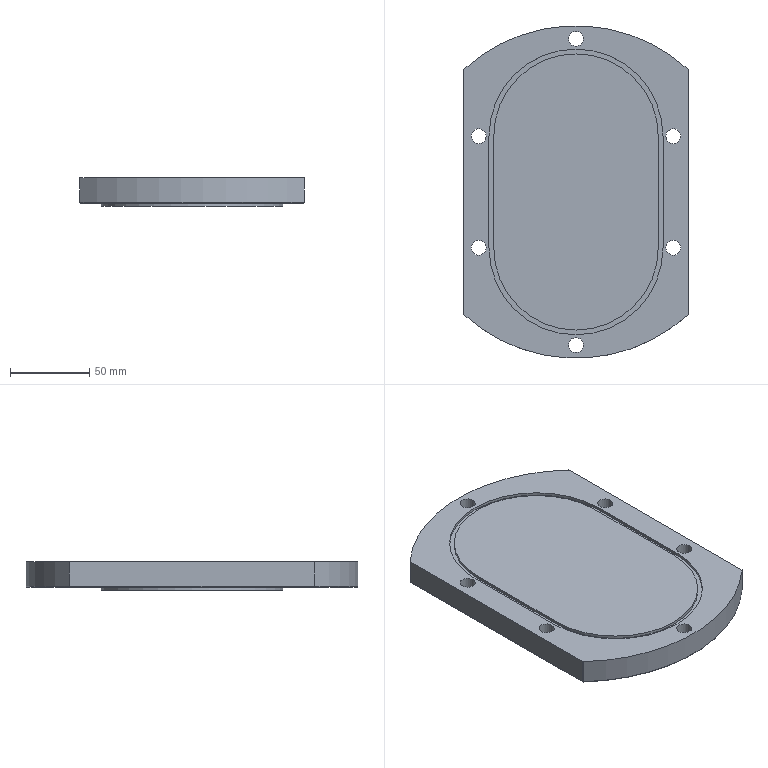CAM job | NX | 3-axis milling, drilling | part box 142 x 210 x 18 mm | stock box 142 x 210 x 23 mm
Tools:
number,name,description,diameter,corner_radius,flute_length,length,flutes
2,D50,Milling Tool-5 Parameters,50.0,0.0,50.0,75.0,2
1,ZXZ,Milling Tool-5 Parameters,6.0,0.0,50.0,75.0,2
9,9.5ZT,Drilling Tool,9.5,0.0,35.0,50.0,2
3,D3,Milling Tool-5 Parameters,3.0,0.0,50.0,75.0,2
5,D25R0.5,Milling Tool-5 Parameters,25.0,0.5,50.0,75.0,2
11,D10JING,Milling Tool-5 Parameters,10.0,0.0,50.0,75.0,2
7,D6A45,Milling Tool-5 Parameters,6.0,0.0,50.0,75.0,2
10,D10,Milling Tool-5 Parameters,10.0,0.0,50.0,75.0,2
Operations:
program,operation,operation_type,tool,method,geometry_group,spindle_rpm,surface_speed,feed_per_tooth,feed_cut,feed_plunge,cut_length_mm,path_length_mm,cut_time_min,machine_time_min
1,FLOOR_WALL_COPY_1,VolumeBased25DMillingOperation,D50,METHOD,A,1200.0,188.0,0.8333,2000.0,1000.0,26924.687,31312.873,13.519,13.958
1,FLOOR_WALL_COPY_COPY,VolumeBased25DMillingOperation,D50,METHOD,A,2500.0,392.0,0.2,1000.0,1000.0,1923.181,1977.181,1.923,1.929
1,DRILLING,Operation,ZXZ,METHOD,A,5000.0,94.0,0.025,250.0,0.0,24.0,613.689,0.096,0.155
1,DRILLING_COPY,Operation,9.5ZT,METHOD,A,2000.0,59.0,0.05,200.0,0.0,149.125,863.938,0.7456,0.8171
1,PLANAR_PROFILE,PlanarMilling,D3,METHOD,A,5000.0,47.0,0.11,1100.0,500.0,17395.215,17451.015,15.934,15.939
1,ZLEVEL_PROFILE_COPY,ZLevelMilling,D25R0.5,METHOD,A,2000.0,157.0,0.55,2200.0,1000.0,17377.191,33790.561,8.509,15.849
1,ZLEVEL_PROFILE_1,ZLevelMilling,D10JING,METHOD,A,5000.0,157.0,0.125,1250.0,100.0,334.594,668.271,0.2677,0.301
1,PLANAR_MILL_COPY_COPY,PlanarMilling,D6A45,METHOD,A,7500.0,141.0,0.0833,1250.0,100.0,1783.471,2799.688,1.427,1.528
2,FLOOR_WALL_COPY_1_COPY,VolumeBased25DMillingOperation,D50,METHOD,B,1200.0,188.0,0.8333,2000.0,1000.0,10979.063,13176.714,5.541,5.761
2,FLOOR_WALL_COPY_COPY_COPY,VolumeBased25DMillingOperation,D50,METHOD,B,2500.0,392.0,0.2,1000.0,1000.0,784.219,838.219,0.7842,0.7896
2,HOLE_MILLING_COPY_COPY,CylinderMilling,D10,METHOD,B,3000.0,94.0,0.3667,2200.0,100.0,3369.429,4200.351,1.532,1.615
2,PLANAR_MILL_COPY_COPY_COPY,PlanarMilling,D6A45,METHOD,B,7500.0,141.0,0.0833,1250.0,100.0,377.197,434.197,0.3018,0.3075
2,PLANAR_MILL_COPY_COPY_COPY_COPY,PlanarMilling,D6A45,METHOD,B,7500.0,141.0,0.0833,1250.0,100.0,898.503,1834.806,0.7188,0.8124